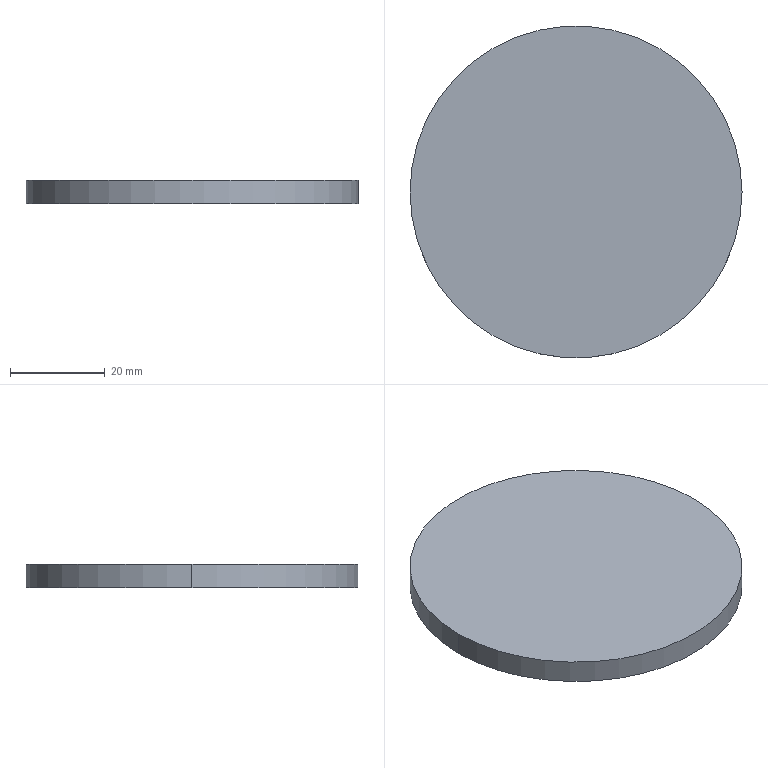Part | STEP file | top cover | 1 solid | 4 faces | box 70 x 70 x 5 mm | volume 19242 mm3 | cylinder 2 | plane 2 | commonest cylinder face diameters 70 x2
STEP:
#1=CARTESIAN_POINT('',(35.,0.,5.));
#2=VERTEX_POINT('',#1);
#3=CARTESIAN_POINT('',(-35.,0.,5.));
#4=VERTEX_POINT('',#3);
#5=CARTESIAN_POINT('',(0.,0.,5.));
#6=DIRECTION('',(0.,0.,1.));
#7=DIRECTION('',(1.,0.,0.));
#8=AXIS2_PLACEMENT_3D('',#5,#6,#7);
#9=CIRCLE('',#8,35.);
#10=EDGE_CURVE('',#2,#4,#9,.T.);
#11=ORIENTED_EDGE('',*,*,#10,.F.);
#12=CARTESIAN_POINT('',(35.,0.,0.));
#13=VERTEX_POINT('',#12);
#14=CARTESIAN_POINT('',(35.,0.,5.));
#15=DIRECTION('',(0.,0.,-1.));
#16=VECTOR('',#15,1000.);
#17=LINE('',#14,#16);
#18=EDGE_CURVE('',#2,#13,#17,.T.);
#19=ORIENTED_EDGE('',*,*,#18,.T.);
#20=CARTESIAN_POINT('',(-35.,0.,0.));
#21=VERTEX_POINT('',#20);
#22=CARTESIAN_POINT('',(0.,0.,0.));
#23=DIRECTION('',(0.,0.,1.));
#24=DIRECTION('',(1.,0.,0.));
#25=AXIS2_PLACEMENT_3D('',#22,#23,#24);
#26=CIRCLE('',#25,35.);
#27=EDGE_CURVE('',#13,#21,#26,.T.);
#28=ORIENTED_EDGE('',*,*,#27,.T.);
#29=CARTESIAN_POINT('',(-35.,0.,5.));
#30=DIRECTION('',(0.,0.,-1.));
#31=VECTOR('',#30,1000.);
#32=LINE('',#29,#31);
#33=EDGE_CURVE('',#4,#21,#32,.T.);
#34=ORIENTED_EDGE('',*,*,#33,.F.);
#35=EDGE_LOOP('',(#11,#19,#28,#34));
#36=FACE_OUTER_BOUND('',#35,.T.);
#37=CARTESIAN_POINT('',(0.,0.,5.));
#38=DIRECTION('',(0.,0.,-1.));
#39=DIRECTION('',(-1.,0.,0.));
#40=AXIS2_PLACEMENT_3D('',#37,#38,#39);
#41=CYLINDRICAL_SURFACE('',#40,35.);
#42=ADVANCED_FACE('',(#36),#41,.T.);
#43=ORIENTED_EDGE('',*,*,#18,.F.);
#44=CARTESIAN_POINT('',(0.,0.,5.));
#45=DIRECTION('',(0.,0.,1.));
#46=DIRECTION('',(1.,0.,0.));
#47=AXIS2_PLACEMENT_3D('',#44,#45,#46);
#48=CIRCLE('',#47,35.);
#49=EDGE_CURVE('',#4,#2,#48,.T.);
#50=ORIENTED_EDGE('',*,*,#49,.F.);
#51=ORIENTED_EDGE('',*,*,#33,.T.);
#52=CARTESIAN_POINT('',(0.,0.,0.));
#53=DIRECTION('',(0.,0.,1.));
#54=DIRECTION('',(1.,0.,0.));
#55=AXIS2_PLACEMENT_3D('',#52,#53,#54);
#56=CIRCLE('',#55,35.);
#57=EDGE_CURVE('',#21,#13,#56,.T.);
#58=ORIENTED_EDGE('',*,*,#57,.T.);
#59=EDGE_LOOP('',(#43,#50,#51,#58));
#60=FACE_OUTER_BOUND('',#59,.T.);
#61=CARTESIAN_POINT('',(0.,0.,5.));
#62=DIRECTION('',(0.,0.,-1.));
#63=DIRECTION('',(-1.,0.,0.));
#64=AXIS2_PLACEMENT_3D('',#61,#62,#63);
#65=CYLINDRICAL_SURFACE('',#64,35.);
#66=ADVANCED_FACE('',(#60),#65,.T.);
#67=ORIENTED_EDGE('',*,*,#49,.T.);
#68=ORIENTED_EDGE('',*,*,#10,.T.);
#69=EDGE_LOOP('',(#67,#68));
#70=FACE_OUTER_BOUND('',#69,.T.);
#71=CARTESIAN_POINT('',(0.,0.,5.));
#72=DIRECTION('',(0.,0.,1.));
#73=DIRECTION('',(1.,0.,0.));
#74=AXIS2_PLACEMENT_3D('',#71,#72,#73);
#75=PLANE('',#74);
#76=ADVANCED_FACE('',(#70),#75,.T.);
#77=ORIENTED_EDGE('',*,*,#57,.F.);
#78=ORIENTED_EDGE('',*,*,#27,.F.);
#79=EDGE_LOOP('',(#77,#78));
#80=FACE_OUTER_BOUND('',#79,.T.);
#81=CARTESIAN_POINT('',(0.,0.,0.));
#82=DIRECTION('',(0.,0.,1.));
#83=DIRECTION('',(1.,0.,0.));
#84=AXIS2_PLACEMENT_3D('',#81,#82,#83);
#85=PLANE('',#84);
#86=ADVANCED_FACE('',(#80),#85,.F.);
#87=CLOSED_SHELL('',(#42,#66,#76,#86));
#88=MANIFOLD_SOLID_BREP('',#87);
#89=CARTESIAN_POINT('',(0.,0.,0.));
#90=DIRECTION('',(0.,0.,1.));
#91=DIRECTION('',(1.,0.,0.));
#92=AXIS2_PLACEMENT_3D('',#89,#90,#91);
#93=(LENGTH_UNIT()NAMED_UNIT(*)SI_UNIT(.MILLI.,.METRE.));
#94=UNCERTAINTY_MEASURE_WITH_UNIT(LENGTH_MEASURE(0.00001),#93,'','');
#95=(NAMED_UNIT(*)PLANE_ANGLE_UNIT()SI_UNIT($,.RADIAN.));
#96=(NAMED_UNIT(*)SI_UNIT($,.STERADIAN.)SOLID_ANGLE_UNIT());
#97=(GEOMETRIC_REPRESENTATION_CONTEXT(3)GLOBAL_UNCERTAINTY_ASSIGNED_CONTEXT((#94))GLOBAL_UNIT_ASSIGNED_CONTEXT((#93,#95,#96))REPRESENTATION_CONTEXT('',''));
#98=ADVANCED_BREP_SHAPE_REPRESENTATION('',(#88,#92),#97);